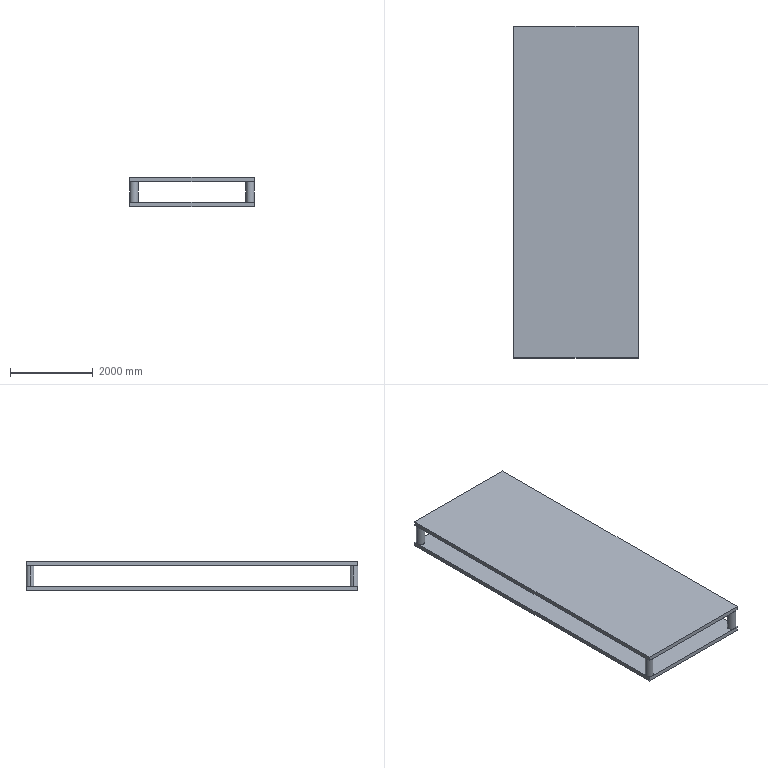Part | STEP file | Truck lifting | 1 solid | 28 faces | box 3000 x 8000 x 700 mm | volume 4862831853 mm3 | plane 20 | cylinder 8 | commonest cylinder face diameters 200 x8